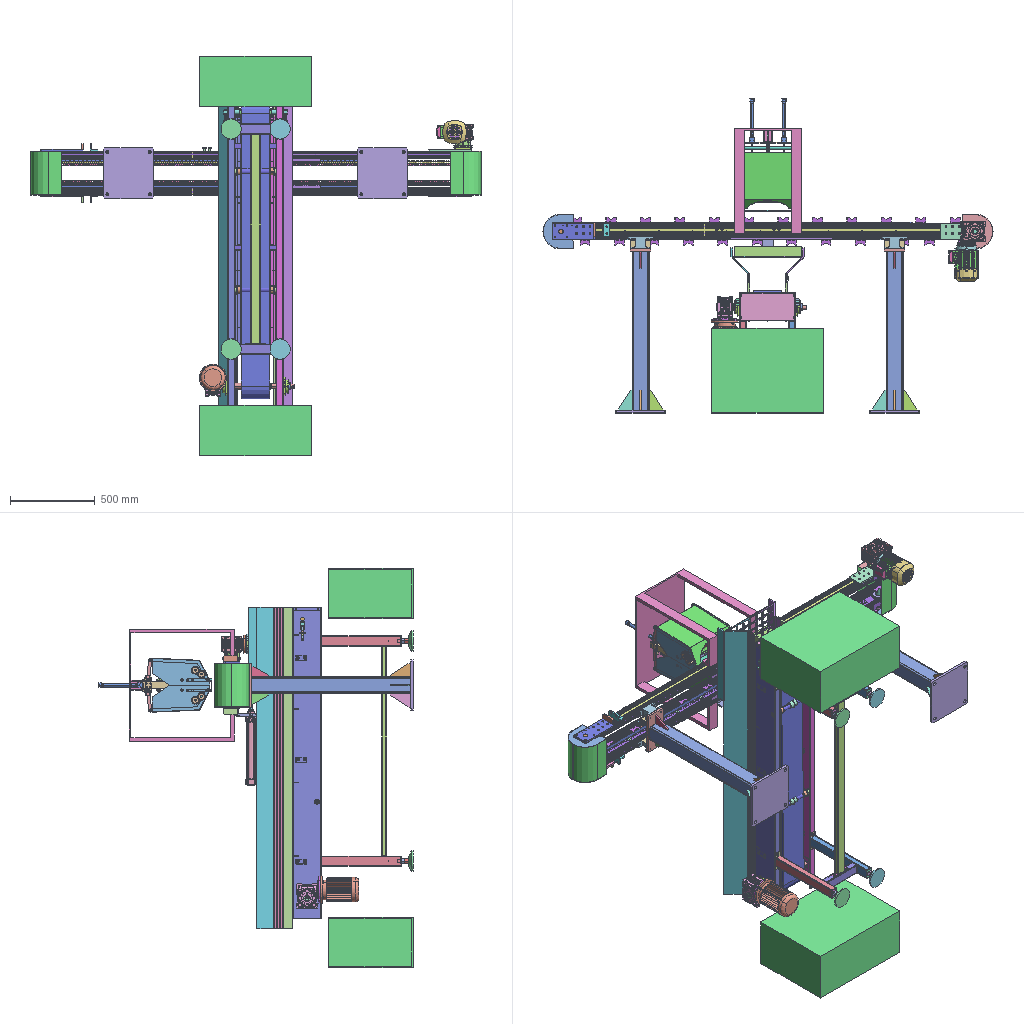Assembly | SolidWorks | 114 different items | 1113 placed | box 2658 x 1857 x 2360 mm
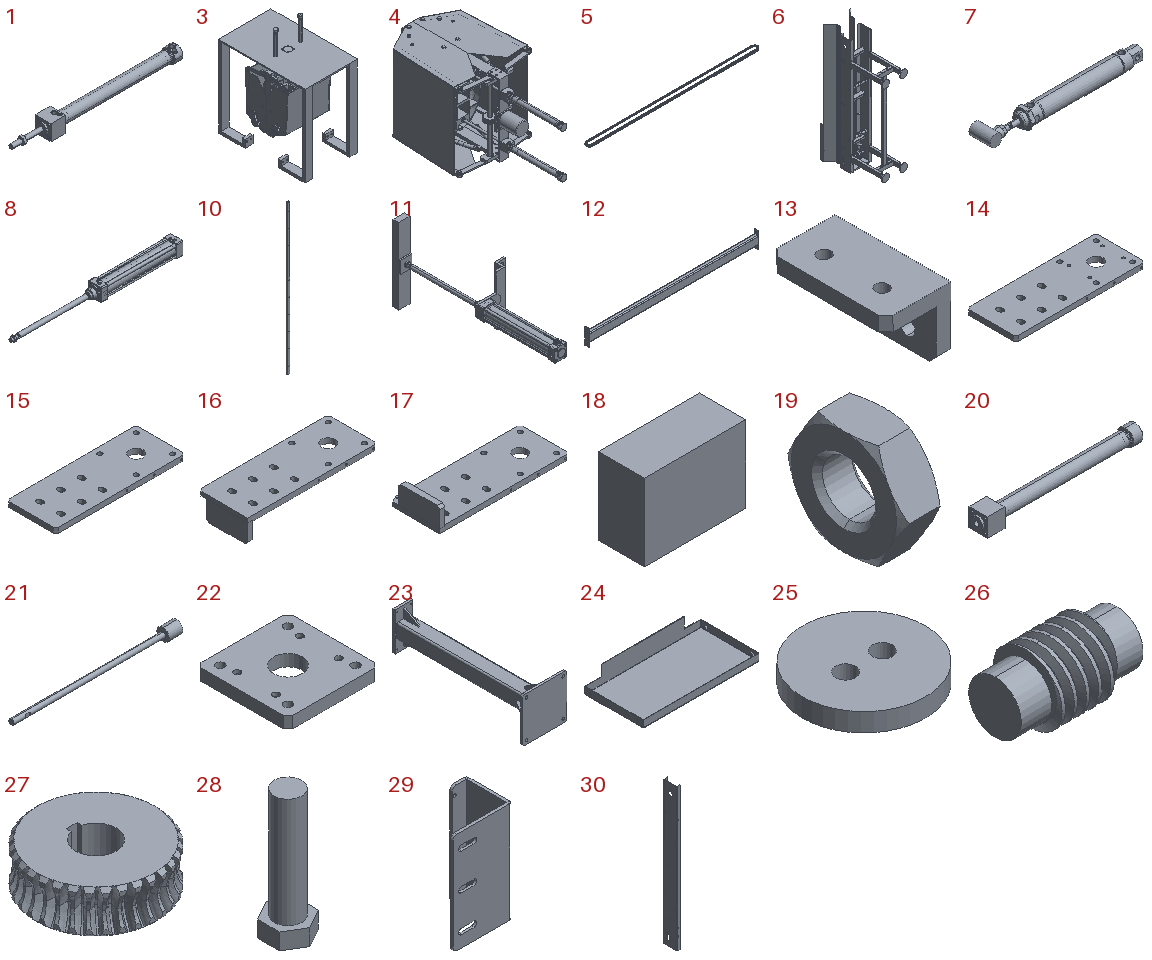Parts list (item | name | quantity | parent item | size | volume | features):
1 | (subassembly) | x2 | in 4 | 322.308 x 30.5 x 30.5 mm | 65420 mm3 | -
2 | (subassembly) | x1 | in 6 | - | - | -
3 | (subassembly) | x1 | - | - | 9842736 mm3 | -
4 | (subassembly) | x1 | in 3 | - | 3212108 mm3 | features CompositeCurve 13, ReferencePattern 9, MirrorCompFeat 4
5 | (subassembly) | x2 | - | - | 534431 mm3 | features ReferencePattern 402, LocalChainPattern 1
6 | (subassembly) | x1 | - | 432 x 974 x 1900 mm | 14530091 mm3 | features ReferencePattern 16, LocalLPattern 2, MirrorCompFeat 2
7 | (subassembly) | x4 | in 4 | 131.292 x 21.537 x 14.5 mm | 12191 mm3 | -
8 | (subassembly) | x1 | in 11 | 828.5 x 86 x 65 mm | 699915 mm3 | -
9 | (subassembly) | x2 | in 6 | - | - | -
10 | (subassembly) | x2 | - | 30 x 24 x 2000 mm | 1183134 mm3 | -
11 | (subassembly) | x1 | - | 190 x 856.5 x 400 mm | 1862385 mm3 | features CompositeCurve 1
12 | - | x1 | in 6 | 1240 x 30 x 120 mm | 613897 mm3 | features ICE 1, MirrorSolid 1, WeldMemberFeat 1, WeldmentFeature 1
13 | - | x2 | - | 45 x 80 x 45 mm | 60593 mm3 | features 3DProfileFeature 2, HoleWzd 2, Chamfer 1, Extrusion 1, LPattern 1
14 | - | x1 | - | 250 x 95 x 10 mm | 222392 mm3 | features 3DProfileFeature 4, HoleWzd 4, ICE 2, LPattern 2, Chamfer 1, Extrusion 1
15 | - | x1 | - | 250 x 95 x 10 mm | 223177 mm3 | features 3DProfileFeature 4, HoleWzd 4, ICE 2, LPattern 2, Chamfer 1, Extrusion 1
16 | - | x1 | - | 250 x 95 x 45 mm | 250777 mm3 | features 3DProfileFeature 4, HoleWzd 4, ICE 4, Chamfer 2, LPattern 2, Extrusion 1
17 | - | x1 | - | 250 x 95 x 45 mm | 250777 mm3 | features 3DProfileFeature 4, HoleWzd 4, ICE 4, Chamfer 2, LPattern 2, Extrusion 1
18 | - | x2 | - | 660 x 300 x 500 mm | 11192000 mm3 | features Extrusion 1, Shell 1
19 | - | x2 | in 1 | 5 x 15.011 x 13 mm | 543.306 mm3 | features BaseBody 1
20 | - | x2 | in 1 | 262 x 30.5 x 30.5 mm | 46248 mm3 | features BaseBody 1
21 | - | x2 | in 1 | 263 x 19.5 x 19.5 mm | 18628 mm3 | features BaseBody 1
22 | - | x1 | - | 95 x 95 x 12 mm | 92833 mm3 | features 3DProfileFeature 3, HoleWzd 3, Chamfer 1, Extrusion 1, ICE 1
23 | - | x2 | - | 300 x 970 x 300 mm | 3763524 mm3 | features Gusset 12, HoleWzd 4, ICE 4, 3DProfileFeature 2, Chamfer 2, MirrorPattern 1, WeldMemberFeat 1, WeldmentFeature 1
24 | - | x1 | in 6 | 324 x 164 x 50 mm | 116232 mm3 | features MoveCopyBody 4, Stock 4, Extrusion 1, FlatPattern 1, FlattenBends 1, ICE 1, ProcessBends 1, Rip 1, SMBaseFlange 1, SheetMetal 1, Shell 1
25 | - | x1 | - | 40 x 40 x 6 mm | 7142 mm3 | features Extrusion 1
26 | - | x1 | in 4 | 39.25 x 22.5 x 22.5 mm | 10547 mm3 | features ICE 2, Helix 1, RefAxis 1, Revolution 1, SweepCut 1
27 | - | x2 | in 4 | 45.721 x 45.721 x 15.75 mm | 18731 mm3 | features CirPattern 1, Cut 1, Helix 1, ICE 1, MirrorPattern 1, RefAxis 1, Revolution 1, SweepCut 1
28 | - | x4 | in 4 | 7.081 x 8.081 x 23 mm | 520.005 mm3 | features Extrusion 1, ICE 1
29 | - | x4 | - | 70 x 54 x 120 mm | 47871 mm3 | features 3DProfileFeature 1, Fillet 1, FlatPattern 1, HoleWzd 1, ICE 1, SMBaseFlange 1, SheetMetal 1
30 | - | x1 | in 6 | 100 x 170 x 1838 mm | 1266311 mm3 | features Cut 1, ICE 1, MirrorStock 1
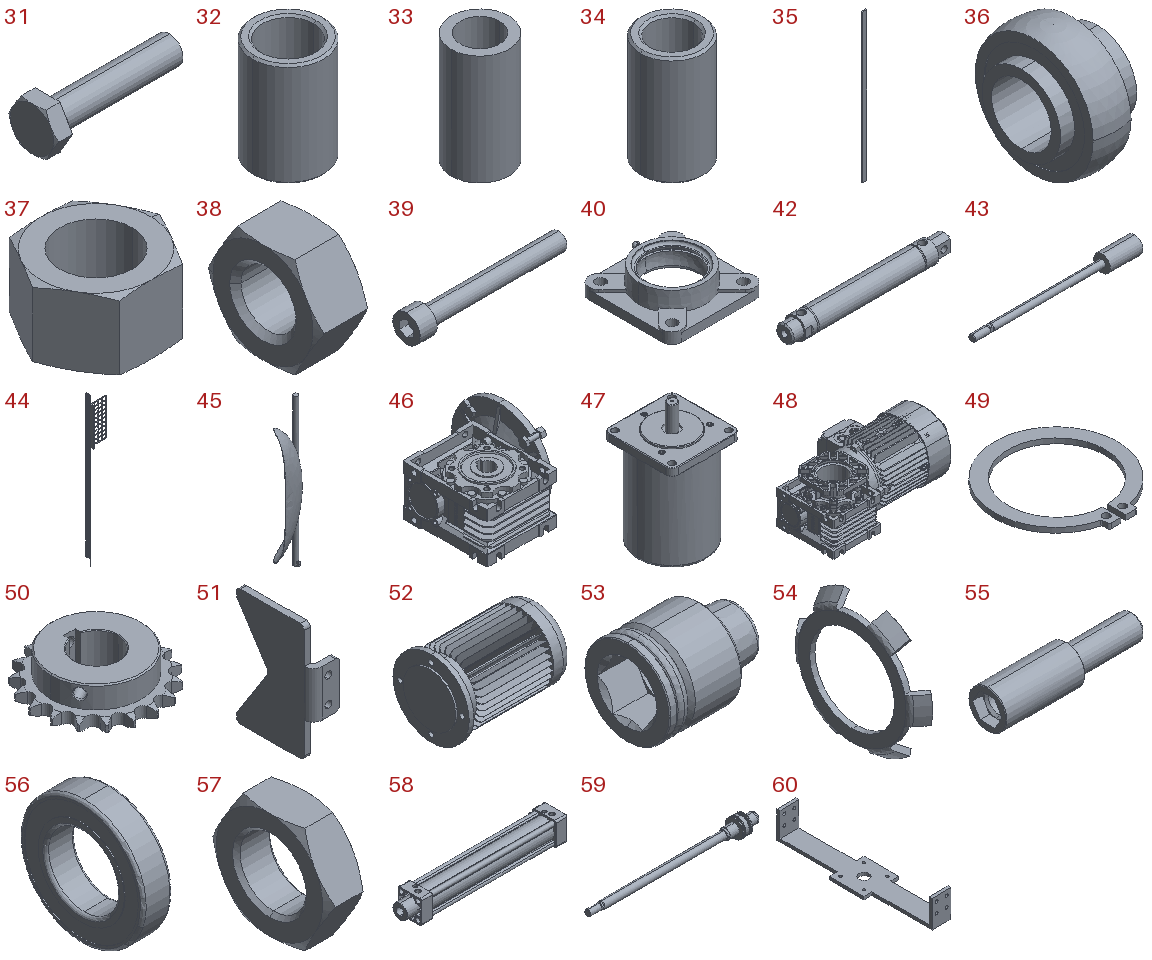31 | - | x4 | - | 51.4 x 18.475 x 16 mm | 4916 mm3 | features RevCut 3, Extrusion 1, Fillet 1, LPattern 1, Revolution 1
32 | - | x1 | in 6 | 35 x 35 x 51 mm | 22832 mm3 | features Chamfer 1, Extrusion 1
33 | - | x4 | in 6 | 30 x 30 x 57 mm | 21477 mm3 | features Chamfer 1, Extrusion 1
34 | - | x4 | in 6 | 30 x 30 x 52 mm | 19435 mm3 | features Chamfer 1, Extrusion 1
35 | - | x2 | - | 55 x 12 x 1900 mm | 1254000 mm3 | features Extrusion 1
36 | - | x2 | - | 38.1 x 62 x 62 mm | 38211 mm3 | features Revolution 3, RevCut 2, CirPattern 1
37 | - | x2 | in 6 | 17.59 x 15.233 x 9.5 mm | 1159 mm3 | features Cut 2, Chamfer 1, Extrusion 1
38 | - | x4 | in 7 | 3 x 6.928 x 6 mm | 65.89 mm3 | features RefAxis 3, 3DProfileFeature 1, ICE 1, Revolution 1, Scale 1
39 | - | x2 | in 6 | 90 x 16 x 16 mm | 8008 mm3 | features BlendCut 1, Cut 1, Fillet 1, LPattern 1, RevCut 1, Revolution 1
40 | - | x2 | - | 108 x 108 x 32.161 mm | 104974 mm3 | features Boss 2, Cut 1, Extrusion 1, RevCut 1, Revolution 1
41 | - | x4 | in 7 | - | - | features RefAxis 3, 3DProfileFeature 1
42 | - | x4 | in 7 | 102.5 x 13.5 x 13.5 mm | 7743 mm3 | features RefAxis 18, 3DProfileFeature 6, ICE 4, RevCut 2, Revolution 1, Scale 1
43 | - | x4 | in 7 | 97.25 x 10 x 10 mm | 2498 mm3 | features RefAxis 6, ICE 4, 3DProfileFeature 2, Revolution 1, Scale 1
44 | - | x1 | in 6 | 216 x 206 x 1900 mm | 3633510 mm3 | features MirrorStock 1
45 | - | x1 | in 4 | 71.359 x 45.899 x 361 mm | 54117 mm3 | features Attribute 3, MirrorStock 1
46 | - | x1 | - | 160 x 190.03 x 160.06 mm | 1157137 mm3 | features BaseBody 9
47 | - | x1 | in 4 | 57 x 57 x 99.8 mm | 207235 mm3 | features ICE 4, CirPattern 1, Fillet 1, LPattern 1, RevCut 1, Revolution 1, Sweep 1
48 | - | x1 | - | - | 1755237 mm3 | features MBimport 1
49 | - | x4 | - | 29.4 x 30.8 x 1.2 mm | 307.898 mm3 | features MBimport 1
50 | - | x4 | - | 83.793 x 83.51 x 22.064 mm | 58564 mm3 | features MBimport 1
51 | - | x39 | - | 13 x 38 x 58 mm | 5478 mm3 | features Fillet 2, ICE 2, FlatPattern 1, HoleWzd 1, SMBaseFlange 1, SheetMetal 1
52 | - | x1 | - | 228.5 x 160 x 160 mm | 2710519 mm3 | features CirPattern 2, ICE 2, Chamfer 1, Fillet 1, Revolution 1
53 | - | x2 | in 8 | 12.8 x 10 x 10 mm | 615.277 mm3 | features BaseBody 1
54 | - | x2 | in 8 | 1.224 x 10 x 9.485 mm | 14.031 mm3 | features BaseBody 1
55 | - | x8 | in 8 | 46 x 12 x 12 mm | 3091 mm3 | features BaseBody 1
56 | - | x8 | in 4 | 5 x 21 x 21 mm | 741.464 mm3 | features BaseBody 16
57 | - | x1 | in 8 | 8 x 26.558 x 23 mm | 2309 mm3 | features BaseBody 1
58 | - | x1 | in 8 | 436.5 x 86 x 65 mm | 489928 mm3 | features BaseBody 1
59 | - | x1 | in 8 | 465.5 x 49.5 x 49.5 mm | 181589 mm3 | features BaseBody 1
60 | - | x1 | in 4 | 70 x 312 x 55 mm | 103168 mm3 | features ICE 4, Cut 1, Extrusion 1
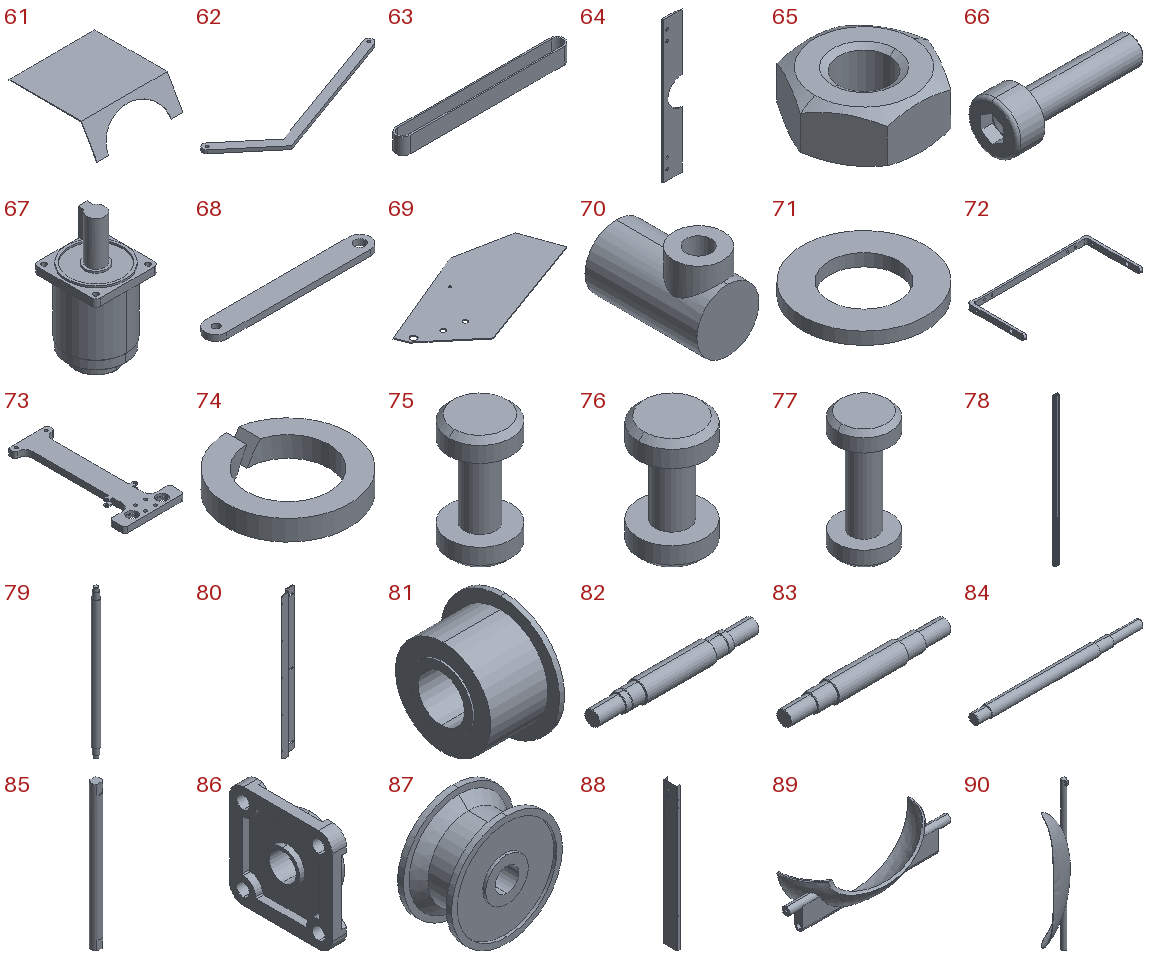61 | - | x2 | in 4 | 328 x 336.732 x 105.923 mm | 222158 mm3 | features Attribute 3, ICE 2, Extrusion 1
62 | - | x4 | in 4 | 377.416 x 116.677 x 7 mm | 52365 mm3 | features Extrusion 1, Fillet 1
63 | - | x1 | - | 1760 x 150 x 170 mm | 9292493 mm3 | features Extrusion 1
64 | - | x2 | in 4 | 37.5 x 3 x 280 mm | 23848 mm3 | features Cut 1, Extrusion 1, ICE 1
65 | - | x2 | - | 8.083 x 7 x 3.2 mm | 104.299 mm3 | features RevCut 2, Chamfer 1, Extrusion 1, LPattern 1
66 | - | x2 | - | 15 x 5.5 x 5.5 mm | 147.329 mm3 | features Fillet 2, RevCut 2, Boss 1, Chamfer 1, Cut 1, Extrusion 1, LPattern 1
67 | - | x2 | in 4 | 35 x 35 x 71 mm | 41626 mm3 | features ICE 7, Fillet 6, Revolution 5, Attribute 3, CirPattern 2, Extrusion 2, Chamfer 1, Dome 1, Emboss 1, LibraryFeature 1, Scale 1
68 | - | x4 | in 4 | 138 x 18 x 5 mm | 11613 mm3 | features ICE 2, Extrusion 1
69 | - | x4 | in 4 | 372.459 x 203.626 x 2 mm | 88439 mm3 | features Cut 6, ICE 4, Extrusion 1, Fillet 1
70 | - | x4 | in 7 | 10 x 18 x 13 mm | 1548 mm3 | features Extrusion 1, ICE 1
71 | - | x3 | - | 16 x 16 x 1.6 mm | 219.911 mm3 | features Extrusion 1
72 | - | x2 | in 4 | 314 x 149.984 x 15 mm | 51932 mm3 | features ICE 3, Fillet 2, Cut 1, Extrusion 1
73 | - | x2 | in 4 | 120 x 255 x 12 mm | 150718 mm3 | features ICE 8, Fillet 2, Cut 1, Extrusion 1
74 | - | x2 | - | 6.6 x 6.6 x 1.1 mm | 20.135 mm3 | features Cut 1, Extrusion 1
75 | - | x4 | in 4 | 12 x 12 x 22 mm | 1265 mm3 | features Chamfer 2, ICE 2, Extrusion 1
76 | - | x4 | in 4 | 12 x 12 x 20 mm | 1208 mm3 | features Chamfer 2, ICE 2, Extrusion 1
77 | - | x4 | in 4 | 12 x 12 x 27 mm | 1406 mm3 | features Chamfer 2, ICE 2, Extrusion 1
78 | - | x2 | - | 80 x 40 x 2300 mm | 2517050 mm3 | features MBimport 1
79 | - | x2 | in 4 | 15 x 15 x 320 mm | 52932 mm3 | features ICE 5, Chamfer 1, Extrusion 1, MirrorPattern 1
80 | - | x2 | - | 70 x 18 x 600 mm | 99365 mm3 | features 3DProfileFeature 1, Fillet 1, FlatPattern 1, HoleWzd 1, ICE 1, SMBaseFlange 1, SheetMetal 1
81 | - | x4 | in 6 | 27.5 x 51 x 51 mm | 16998 mm3 | features Revolution 1
82 | - | x1 | - | 276 x 35 x 35 mm | 204867 mm3 | features ICE 4, Chamfer 3, 3DProfileFeature 1, HoleWzd 1, MirrorPattern 1, Revolution 1
83 | - | x1 | - | 276 x 35 x 35 mm | 205103 mm3 | features Chamfer 1, ICE 1, Revolution 1
84 | - | x1 | - | 511 x 35 x 35 mm | 419085 mm3 | features ICE 2, Chamfer 1, HoleWzd 1, Revolution 1
85 | - | x1 | in 6 | 25 x 25 x 374 mm | 180094 mm3 | features ICE 2, Chamfer 1, Extrusion 1, MirrorPattern 1
86 | - | x4 | - | 35.7 x 95 x 95 mm | 103360 mm3 | features MBimport 1
87 | - | x4 | in 6 | 117 x 57 x 117 mm | 342775 mm3 | features ICE 2, MirrorPattern 1, Revolution 1
88 | - | x1 | in 6 | 100 x 170 x 1838 mm | 1271220 mm3 | features ICE 5, MoveCopyBody 4, Stock 4, FlatPattern 2, SMBaseFlange 2, SheetMetal 2, Chamfer 1, HoleWzd 1, LPattern 1, RefAxis 1, SMMiteredFlange 1
89 | - | x2 | in 4 | 328 x 89.443 x 98.481 mm | 199314 mm3 | features ICE 3, MirrorPattern 2, 3DProfileFeature 1, Attribute 1, Chamfer 1, Revolution 1
90 | - | x1 | in 4 | 71.359 x 45.899 x 361 mm | 54038 mm3 | features ICE 4, Attribute 3, Cut 3, Chamfer 2, ExtruThin 1, Fillet 1, Shell 1, Sweep 1
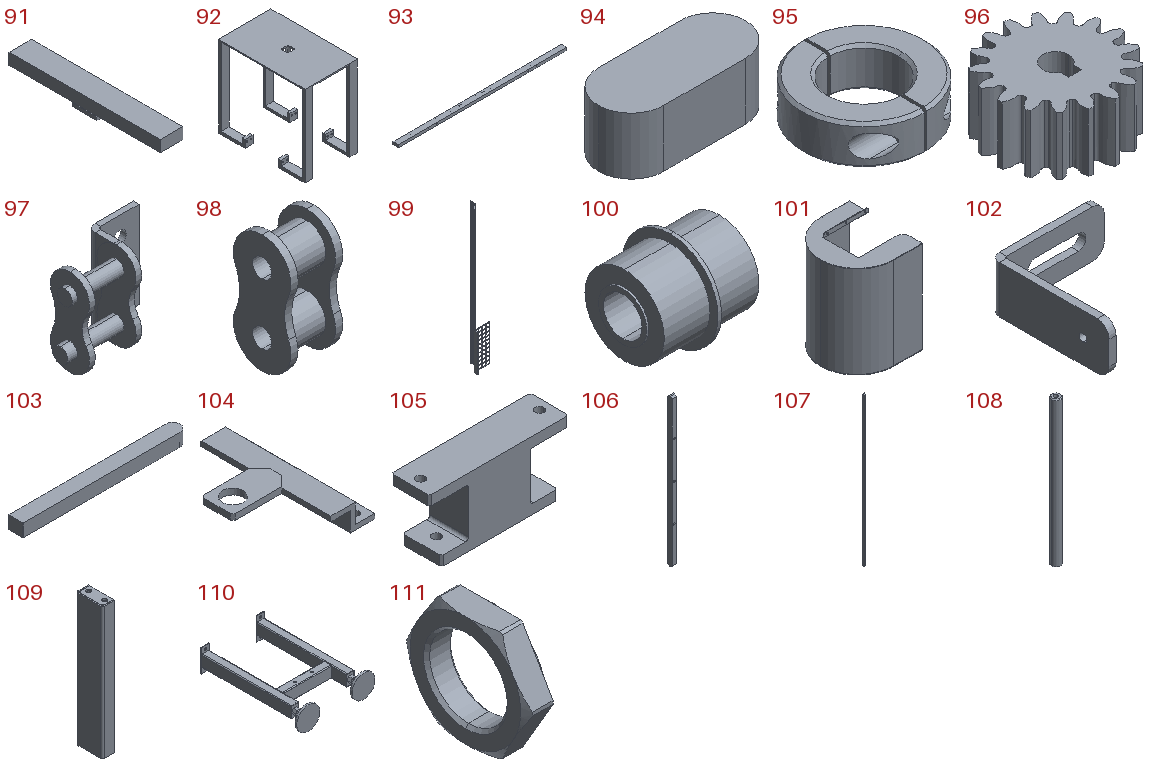91 | - | x1 | in 11 | 60 x 400 x 40 mm | 758635 mm3 | features Cut 2, ICE 2, Chamfer 1, Extrusion 1, HoleWzd 1
92 | - | x1 | in 3 | 400 x 660 x 620 mm | 6630473 mm3 | features MirrorPattern 6, ICE 5, Cut 1, Extrusion 1
93 | - | x2 | - | 2544 x 80 x 40 mm | 8091371 mm3 | features Cut 4, Extrusion 1, LPattern 1
94 | - | x4 | - | 18 x 8 x 7 mm | 911.858 mm3 | features MBimport 1
95 | - | x2 | in 6 | 44 x 43.989 x 14 mm | 11608 mm3 | features ICE 3, Chamfer 1, Extrusion 1, MirrorSolid 1
96 | - | x4 | in 4 | 47.423 x 47.235 x 22.5 mm | 29237 mm3 | features Attribute 3, ICE 2, CirPattern 1, Cut 1, Extrusion 1, RefAxis 1, Scale 1
97 | - | x404 | in 5 | 27.296 x 13.105 x 23.11 mm | 1387 mm3 | features MoveFace 9, 3DProfileFeature 1, BaseBody 1, EdgeFlange 1, FlatPattern 1, HoleWzd 1, SMBaseFlange 1, SheetMetal 1
98 | - | x404 | in 5 | 10.85 x 12.07 x 24.77 mm | 1258 mm3 | features MoveFace 4, BaseBody 1, DelFace 1
99 | - | x1 | in 6 | 216 x 206 x 1900 mm | 3633510 mm3 | features ICE 5, Cut 1, Extrusion 1, LPattern 1
100 | - | x2 | in 6 | 51 x 49.5 x 49.5 mm | 50740 mm3 | features Revolution 1
101 | - | x2 | - | 182 x 204 x 280 mm | 308459 mm3 | features FlatPattern 3, SMBaseFlange 2, SheetMetal 2, 3DProfileFeature 1, EdgeFlange 1, Fillet 1, HoleWzd 1, MirrorSolid 1
102 | - | x20 | - | 45 x 50 x 20 mm | 4913 mm3 | features 3DProfileFeature 1, Fillet 1, FlatPattern 1, HoleWzd 1, ICE 1, SMBaseFlange 1, SheetMetal 1
103 | - | x1 | - | 90 x 8 x 7 mm | 4991 mm3 | features MBimport 1
104 | - | x1 | in 11 | 190 x 265 x 52 mm | 403840 mm3 | features ICE 4, Chamfer 2, Extrusion 1
105 | - | x4 | - | 144 x 40 x 70 mm | 231204 mm3 | features ICE 4, 3DProfileFeature 3, HoleWzd 3, Cut 2, Chamfer 1, Extrusion 1, Fillet 1, MirrorPattern 1
106 | - | x4 | - | 6 x 6 x 200 mm | 7064 mm3 | features 3DProfileFeature 1, Chamfer 1, Extrusion 1, HoleWzd 1
107 | - | x2 | - | 6 x 6 x 600 mm | 21405 mm3 | features 3DProfileFeature 1, Chamfer 1, Extrusion 1, HoleWzd 1
108 | - | x2 | in 6 | 20 x 20 x 324 mm | 98619 mm3 | features HoleWzd 2, Chamfer 1, Extrusion 1
109 | - | x3 | in 6 | 30 x 65 x 324 mm | 129406 mm3 | features MoveCopyBody 5, Stock 5, FlatPattern 2, SMBaseFlange 2, SheetMetal 2, ICE 1, MirrorSolid 1
110 | - | x2 | in 6 | 410 x 543 x 120 mm | 1073407 mm3 | features MoveCopyBody 4, Stock 4, ICE 3, WeldMemberFeat 2, HoleWzd 1, MirrorSolid 1, WeldCornerFeat 1, WeldmentFeature 1
111 | - | x4 | in 7 | 3.5 x 16.5 x 14.5 mm | 336.894 mm3 | features RefAxis 6, 3DProfileFeature 2, ICE 1, RevCut 1, Revolution 1, Scale 1
112 | VSW26-40-L2000-K10-P200.stp (subassembly) | x1 | - | - | - | -
113 | _VSW26-40                                                        40 2000 10 200 VSW26.stp | x1 | - | - | - | -
114 | _VSW26-L2000                                                        40 2000 10 200 VSW26.stp | x1 | - | - | - | -
Mates (type | each side: item.copy, entity, surface, feature), first 366 of 395 lines:
In the top assembly
Coincident | 23.1 face plane Boss-Extrude 1 | 23.2 face plane Boss-Extrude 1
Coincident | 23.1 face plane Square Tube 100 X 100 X 5(1) | 23.2 face plane Square Tube 100 X 100 X 5(1)
DistanceDim | 23.2 face plane Square Tube 100 X 100 X 5(1) | 23.1 face plane Square Tube 100 X 100 X 5(1)
Concentric | 105.1 face cylinder M8 Clearance Hole 1 | 23.1 face cylinder M8 Tapped Hole 1 | 2 times
Coincident | 105.1 face plane Boss-Extrude 1 | 23.1 face plane Boss-Extrude 2
Concentric | 23.1 face cylinder M8 Tapped Hole 1 | 105.2 face cylinder M8 Clearance Hole 1 | 2 times
Coincident | 23.1 face plane Boss-Extrude 2 | 105.2 face plane Boss-Extrude 1
Concentric | 23.2 face cylinder M8 Tapped Hole 1 | 105.3 face cylinder M8 Clearance Hole 1 | 2 times
Coincident | 23.2 face plane Boss-Extrude 2 | 105.3 face plane Boss-Extrude 1
Concentric | 23.2 face cylinder M8 Tapped Hole 1 | 105.4 face cylinder M8 Clearance Hole 1 | 2 times
Coincident | 23.2 face plane Boss-Extrude 2 | 105.4 face plane Boss-Extrude 1
Coincident | 105.1 face plane Boss-Extrude 1 | 78.1 face plane AOB05-4080E-L2300.stp
Coincident | 78.2 face plane AOB05-4080E-L2300.stp | 78.1 face plane AOB05-4080E-L2300.stp | 2 times
Width | 78.1 face plane AOB05-4080E-L2300.stp | 78.1 face plane AOB05-4080E-L2300.stp | 105.1 face plane Boss-Extrude 1 | 105.1 face plane Boss-Extrude 1
Width | 78.2 face plane AOB05-4080E-L2300.stp | 78.2 face plane AOB05-4080E-L2300.stp | 105.2 face plane Boss-Extrude 1 | 105.2 face plane Boss-Extrude 1
Width | 78.2 face plane AOB05-4080E-L2300.stp | 78.2 face plane AOB05-4080E-L2300.stp | 23.1 face plane Square Tube 100 X 100 X 5(1) | 23.2 face plane Square Tube 100 X 100 X 5(1)
Coincident | 15.1 face plane Boss-Extrude 1 | 78.2 face plane AOB05-4080E-L2300.stp | 2 times
Concentric | 15.1 face cylinder Cut-Extrude 5 | 86.1 face cylinder BDR-205.stp
Coincident | 15.1 face plane Boss-Extrude 1 | 86.1 face plane BDR-205.stp
Width | 78.1 face plane AOB05-4080E-L2300.stp | 78.2 face plane AOB05-4080E-L2300.stp | 50.1 face plane VLF02-40-19-D30.stp | 50.2 face plane VLF02-40-19-D30.stp
Concentric | 86.1 face cylinder BDR-205.stp | 83.1 face cylinder Revolve 1 | 2 times
Coincident | 83.1 face plane Revolve 1 | 50.2 face plane VLF02-40-19-D30.stp
Concentric | 83.1 face cylinder Revolve 1 | 50.2 face cylinder VLF02-40-19-D30.stp
Concentric | 83.1 face cylinder Revolve 1 | 50.1 face cylinder VLF02-40-19-D30.stp
Coincident | 83.1 face plane Revolve 1 | 50.1 face plane VLF02-40-19-D30.stp
Concentric | 83.1 face cylinder Cut-Extrude 1 | 94.1 face cylinder BLC01-B8-L18.stp
Coincident | 83.1 face plane Cut-Extrude 1 | 94.1 face plane BLC01-B8-L18.stp | 2 times
Concentric | 83.1 face cylinder Cut-Extrude 1 | 94.2 face cylinder BLC01-B8-L18.stp
Coincident | 83.1 face plane Cut-Extrude 1 | 94.2 face plane BLC01-B8-L18.stp | 2 times
Coincident | 50.2 face plane VLF02-40-19-D30.stp | 94.2 face plane BLC01-B8-L18.stp
Coincident | 50.1 face plane VLF02-40-19-D30.stp | 94.1 face plane BLC01-B8-L18.stp
DistanceDim | 15.1 face plane Boss-Extrude 1 | 78.2 face plane AOB05-4080E-L2300.stp
Coincident | 78.1 face plane AOB05-4080E-L2300.stp | 14.1 face plane Boss-Extrude 1 | 2 times
Coincident | 15.1 face plane Boss-Extrude 1 | 14.1 face plane Boss-Extrude 1
Concentric | 86.2 face cylinder BDR-205.stp | 14.1 face cylinder Cut-Extrude 5
Coincident | 86.2 face plane BDR-205.stp | 14.1 face plane Boss-Extrude 1
Concentric | 22.1 face cylinder Cut-Extrude 1 | 14.1 face cylinder Cut-Extrude 5
Coincident | 22.1 face plane Boss-Extrude 1 | 14.1 face plane Boss-Extrude 1
Parallel | 22.1 face plane Boss-Extrude 1 | 14.1 face plane Boss-Extrude 1
Coincident | 78.1 face plane AOB05-4080E-L2300.stp | 17.1 face plane Boss-Extrude 1 | 2 times
DistanceDim | 17.1 face plane Boss-Extrude 1 | 78.1 face plane AOB05-4080E-L2300.stp
Coincident | 78.2 face plane AOB05-4080E-L2300.stp | 16.1 face plane Boss-Extrude 1 | 2 times
Coincident | 17.1 face plane Boss-Extrude 1 | 16.1 face plane Boss-Extrude 1
Coincident | 13.1 face plane Boss-Extrude 1 | 78.1 face plane AOB05-4080E-L2300.stp | 2 times
DistanceDim | 13.1 face plane Boss-Extrude 1 | 17.1 face plane Boss-Extrude 1
Concentric | 17.1 face cylinder Cut-Extrude 5 | 86.3 face cylinder BDR-205.stp
Coincident | 17.1 face plane Boss-Extrude 1 | 86.3 face plane BDR-205.stp
Coincident | 16.1 face plane Boss-Extrude 1 | 86.4 face plane BDR-205.stp
Concentric | 16.1 face cylinder Cut-Extrude 5 | 86.4 face cylinder BDR-205.stp
Concentric | 86.4 face cylinder BDR-205.stp | 82.1 face cylinder Revolve 1
Concentric | 82.1 face cylinder Revolve 1 | 50.3 face cylinder VLF02-40-19-D30.stp
Concentric | 82.1 face cylinder Revolve 1 | 50.4 face cylinder VLF02-40-19-D30.stp
Concentric | 82.1 face cylinder Cut-Extrude 1 | 94.3 face cylinder BLC01-B8-L18.stp
Coincident | 82.1 face plane Cut-Extrude 1 | 94.3 face plane BLC01-B8-L18.stp
Concentric | 82.1 face cylinder Cut-Extrude 1 | 94.4 face cylinder BLC01-B8-L18.stp
Coincident | 82.1 face plane Cut-Extrude 1 | 94.4 face plane BLC01-B8-L18.stp
Coincident | 82.1 face plane Revolve 1 | 50.3 face plane VLF02-40-19-D30.stp
Coincident | 82.1 face plane Revolve 1 | 50.4 face plane VLF02-40-19-D30.stp
Width | 50.3 face plane VLF02-40-19-D30.stp | 50.4 face plane VLF02-40-19-D30.stp | 78.1 face plane AOB05-4080E-L2300.stp | 78.2 face plane AOB05-4080E-L2300.stp
Concentric | 50.4 face cylinder VLF02-40-19-D30.stp | 5.1 select_type:24
Width | 98.1 face plane Import 1 | 98.1 face plane Import 1 | 50.4 face plane VLF02-40-19-D30.stp | 50.4 face plane VLF02-40-19-D30.stp
Concentric | 50.2 face cylinder VLF02-40-19-D30.stp | 5.2 select_type:24
Coincident | 97.1 face plane Edge-Flange 1 | 51.1 face plane Base-Flange 1
Parallel | 78.2 face plane AOB05-4080E-L2300.stp | 5.2 select_type:24
Width | 98.2 face plane Import 1 | 98.2 face plane Import 1 | 50.3 face plane VLF02-40-19-D30.stp | 50.3 face plane VLF02-40-19-D30.stp
Parallel | 78.1 face plane AOB05-4080E-L2300.stp | 5.1 select_type:24
Concentric | 97.2 face cylinder Ø3.4 (3.4) DiameterHole 1 | 51.2 face cylinder Ø3.4 (3.4) DiameterHole 1 | 2 times
Coincident | 97.2 face plane Edge-Flange 1 | 51.2 face plane Base-Flange 1
Concentric | 97.3 face cylinder Ø3.4 (3.4) DiameterHole 1 | 51.3 face cylinder Ø3.4 (3.4) DiameterHole 1 | 2 times
Coincident | 97.3 face plane Edge-Flange 1 | 51.3 face plane Base-Flange 1
Coincident | 29.1 face plane Base-Flange 1 | 23.1 face plane Boss-Extrude 2
Width | 29.1 face plane Base-Flange 1 | 29.1 face plane Base-Flange 1 | 23.1 face plane Boss-Extrude 2 | 23.1 face plane Boss-Extrude 2
Coincident | 29.1 face plane Base-Flange 1 | 29.2 face plane Base-Flange 1 | 2 times
Width | 29.2 face plane Base-Flange 1 | 29.1 face plane Base-Flange 1 | 23.1 face plane Boss-Extrude 2 | 23.1 face plane Boss-Extrude 2
Coincident | 29.3 face plane Base-Flange 1 | 29.4 face plane Base-Flange 1 | 2 times
Coincident | 23.2 face plane Boss-Extrude 2 | 29.3 face plane Base-Flange 1
Coincident | 16.1 face plane Boss-Extrude 1 | 101.1 face plane Mirror 1
DistanceDim | 16.1 face plane Boss-Extrude 1 | 101.1 face plane Mirror 1
Width | 101.1 face plane Mirror 1 | 101.1 face plane Base-Flange 2 | 17.1 face plane Boss-Extrude 1 | 16.1 face plane Boss-Extrude 1
Coincident | 14.1 face plane Boss-Extrude 1 | 101.2 face plane Mirror 1
DistanceDim | 14.1 face plane Boss-Extrude 1 | 101.2 face plane Mirror 1
Coincident | 101.2 face plane Mirror 1 | 101.1 face plane Base-Flange 2
Concentric | 22.1 face cylinder Cut-Extrude 1 | 48.1 face cylinder NMRW050-MS7124-B14-FA1-D25.STEP
Parallel | 22.1 face plane Boss-Extrude 1 | 48.1 face plane NMRW050-MS7124-B14-FA1-D25.STEP
Coincident | 22.1 face plane Boss-Extrude 1 | 48.1 face plane NMRW050-MS7124-B14-FA1-D25.STEP
Coincident | 97.4 face plane Edge-Flange 1 | 51.4 face plane Base-Flange 1
Concentric | 97.1 face cylinder Ø3.4 (3.4) DiameterHole 1 | 51.1 face cylinder Ø3.4 (3.4) DiameterHole 1 | 2 times
Concentric | 97.5 face cylinder Ø3.4 (3.4) DiameterHole 1 | 51.4 face cylinder Ø3.4 (3.4) DiameterHole 1 | 2 times
Coincident | 78.2 face plane AOB05-4080E-L2300.stp | 13.2 face plane Boss-Extrude 1
Coincident | 13.1 face plane Boss-Extrude 1 | 13.2 face plane Boss-Extrude 1
Concentric | 82.1 face cylinder Mirror 1 | 49.1 face cylinder TBP01-25.stp
Coincident | 82.1 face plane Mirror 1 | 49.1 face plane TBP01-25.stp
Concentric | 82.1 face cylinder Cut-Extrude 3 | 49.2 face cylinder TBP01-25.stp
Coincident | 82.1 face plane Cut-Extrude 3 | 49.2 face plane TBP01-25.stp
Concentric | 97.6 face cylinder Ø3.4 (3.4) DiameterHole 1 | 51.5 face cylinder Ø3.4 (3.4) DiameterHole 1 | 2 times
Coincident | 97.6 face plane Edge-Flange 1 | 51.5 face plane Base-Flange 1
Concentric | 97.7 face cylinder Ø3.4 (3.4) DiameterHole 1 | 51.6 face cylinder Ø3.4 (3.4) DiameterHole 1 | 2 times
Coincident | 97.7 face plane Edge-Flange 1 | 51.6 face plane Base-Flange 1
Coincident | 78.1 face plane AOB05-4080E-L2300.stp | 102.1 face plane Base-Flange 1
Coincident | 78.2 face plane AOB05-4080E-L2300.stp | 102.2 face plane Base-Flange 1
Coincident | 29.1 face plane Base-Flange 1 | 106.1 face plane Boss-Extrude 1 | 2 times
Concentric | 29.1 face cylinder M3 Clearance Hole 1 | 106.1 face cylinder M3 Tapped Hole 1
Coincident | 29.2 face plane Base-Flange 1 | 106.2 face plane Boss-Extrude 1 | 2 times
Concentric | 29.2 face cylinder M3 Clearance Hole 1 | 106.2 face cylinder M3 Tapped Hole 1
Width | 106.1 face plane Boss-Extrude 1 | 106.1 face plane Boss-Extrude 1 | 98.3 face plane Import 1 | 98.3 face plane Import 1
Coincident | 29.3 face plane Base-Flange 1 | 106.3 face plane Boss-Extrude 1 | 2 times
Concentric | 29.3 face cylinder M3 Clearance Hole 1 | 106.3 face cylinder M3 Tapped Hole 1
Coincident | 29.4 face plane Base-Flange 1 | 106.4 face plane Boss-Extrude 1 | 2 times
Concentric | 29.4 face cylinder M3 Clearance Hole 1 | 106.4 face cylinder M3 Tapped Hole 1
Coincident | 29.1 face plane Base-Flange 1 | 29.3 face plane Base-Flange 1
Width | 29.3 face plane Base-Flange 1 | 29.3 face plane Base-Flange 1 | 23.2 face plane Boss-Extrude 2 | 23.2 face plane Boss-Extrude 2
Coincident | 29.2 face plane Base-Flange 1 | 29.4 face plane Base-Flange 1
Coincident | 80.1 face plane Base-Flange 1 | 107.1 face plane Boss-Extrude 1 | 2 times
Concentric | 80.1 face cylinder M3 Clearance Hole 1 | 107.1 face cylinder M3 Tapped Hole 1
Coincident | 78.2 face plane AOB05-4080E-L2300.stp | 80.1 face plane Base-Flange 1
Coincident | 106.4 face plane Boss-Extrude 1 | 107.1 face plane Boss-Extrude 1
Coincident | 80.2 face plane Base-Flange 1 | 107.2 face plane Boss-Extrude 1 | 2 times
Concentric | 80.2 face cylinder M3 Clearance Hole 1 | 107.2 face cylinder M3 Tapped Hole 1
Coincident | 80.1 face plane Base-Flange 1 | 80.2 face plane Base-Flange 1 | 2 times
Coincident | 106.3 face plane Boss-Extrude 1 | 107.2 face plane Boss-Extrude 1
Concentric | 105.1 face cylinder Mirror 2 | 71.1 face cylinder Base-Extrude
Coincident | 105.1 face plane Cut-Extrude 2 | 71.1 face plane Base-Extrude
Concentric | 105.1 face cylinder Mirror 2 | 74.1 face cylinder Base-Extrude
Coincident | 71.1 face plane Base-Extrude | 74.1 face plane Base-Extrude
Concentric | 51.7 face cylinder Ø3.4 (3.4) DiameterHole 1 | 71.2 face cylinder Base-Extrude
Coincident | 51.7 face plane Base-Flange 1 | 71.2 face plane Base-Extrude
Concentric | 51.7 face cylinder Ø3.4 (3.4) DiameterHole 1 | 74.2 face cylinder Base-Extrude
Coincident | 71.2 face plane Base-Extrude | 74.2 face plane Base-Extrude
Coincident | 51.7 face plane Base-Flange 1 | 65.1 face plane BaseNut
Concentric | 74.2 face cylinder Base-Extrude | 65.2 face cone EndChamfer
Coincident | 74.2 face plane Base-Extrude | 65.2 face plane BaseNut
Concentric | 51.7 face cylinder Base Bend 1 | 66.1 face cylinder BaseBody
Concentric | 51.7 face cylinder Ø3.4 (3.4) DiameterHole 1 | 66.2 face cylinder BaseBody
Coincident | 71.3 face plane Base-Extrude | 66.2 face plane BaseHead
Coincident | 97.8 face plane Edge-Flange 1 | 71.3 face plane Base-Extrude
Concentric | 66.2 face cylinder BaseHead | 71.3 face cylinder Base-Extrude
Coincident | 102.3 face plane Base-Flange 1 | 93.1 face plane Boss-Extrude 1
Coincident | 102.1 face plane Base-Flange 1 | 93.1 face plane Boss-Extrude 1 | 2 times
Coincident | 101.1 face plane Base-Flange 2 | 93.1 face plane Boss-Extrude 1
Coincident | 23.2 face plane Boss-Extrude 1 | 110.1 face plane M20 Foot | 2 times
Coincident | 23.1 face plane Boss-Extrude 1 | 18.1 face plane Boss-Extrude 1
Parallel | 24.1 face plane Boss-Extrude 1 | 18.1 face plane Boss-Extrude 1
DistanceDim | 110.1 face plane Structure Member 1 | 18.1 face plane Boss-Extrude 1
Concentric | 84.1 face cylinder Revolve 1 | 36.1 face sphere Boss-Revolve 3
Concentric | 84.1 face cylinder Revolve 1 | 40.1 edge
Coincident | 88.1 face plane Base-Flange 1 | 40.1 face plane Base-Extrude
Concentric | 84.1 face cylinder Revolve 1 | 36.2 face cylinder Boss-Revolve 3
Coincident | 40.1 face plane Cut-Revolve 1 | 36.2 face plane Boss-Revolve 3
Concentric | 84.1 face cylinder Revolve 1 | 46.1 edge
Parallel | 88.1 face plane Base-Flange 1 | 46.1 face plane Import 1
Coincident | 46.1 face plane Import 7 | 25.1 face plane Boss-Extrude 1
Concentric | 46.1 edge | 25.1 edge
Concentric | 46.1 edge | 52.1 face cylinder Revolve 1
Concentric | 46.1 face cylinder Import 9 | 52.1 edge
Coincident | 46.1 face plane Import 9 | 52.1 face plane Revolve 1
DistanceDim | 84.1 face plane Revolve 1 | 36.1 face plane Boss-Revolve 3
Width | 18.1 face plane Boss-Extrude 1 | 18.1 face plane Boss-Extrude 1 | 30.1 face plane Side Beam 3 Mirror | 88.1 face plane Base-Flange 1
Concentric | 84.1 face cylinder Revolve 1 | 87.1 face cylinder Cut-Extrude 1
Coincident | 87.2 face plane Revolve 1 | 87.1 face plane Revolve 1
Concentric | 84.1 face cylinder Revolve 1 | 87.3 edge
Coincident | 87.4 face plane Revolve 1 | 87.3 face plane Revolve 1
Concentric | 30.1 edge | 84.1 face cylinder Revolve 1
Concentric | 84.1 face cylinder Revolve 1 | 40.2 edge
Coincident | 30.1 face plane Side Beam 3 Mirror | 40.2 face plane Base-Extrude
Parallel | 30.1 face plane Side Beam 3 Mirror | 40.2 face plane Base-Extrude
Concentric | 84.1 face cylinder Revolve 1 | 63.1 edge
Width | 63.1 face plane Boss-Extrude 1 | 63.1 face plane Boss-Extrude 1 | 30.1 face plane Side Beam 3 Mirror | 88.1 face plane Base-Flange 1
Coincident | 44.1 face plane Large C Type Guardrail_Mirror | 35.1 face plane Boss-Extrude 1 | 3 times
Coincident | 99.1 face plane Boss-Extrude 2 | 35.2 face plane Boss-Extrude 1 | 2 times
Coincident | 35.1 face plane Boss-Extrude 1 | 35.2 face plane Boss-Extrude 1
Width | 92.1 face plane Boss-Extrude 1 | 92.1 face plane Boss-Extrude 1 | 101.2 face plane Mirror 1 | 101.1 face plane Base-Flange 2
Width | 92.1 face plane Boss-Extrude 1 | 92.1 face plane Boss-Extrude 1 | 17.1 face plane Boss-Extrude 1 | 16.1 face plane Boss-Extrude 1
Width | 23.2 face plane Square Tube 100 X 100 X 5(1) | 23.1 face plane Square Tube 100 X 100 X 5(1) | 88.1 face plane Base-Flange 1 | 30.1 face plane Side Beam 3 Mirror
Coincident | 102.1 face plane Base-Flange 1 | 102.2 face plane Base-Flange 1
DistanceDim | 102.2 face plane Base-Flange 1 | 15.1 face plane Boss-Extrude 1
Width | 104.1 face plane Boss-Extrude 2 | 104.1 face plane Boss-Extrude 2 | 92.1 face plane Boss-Extrude 1 | 92.1 face plane Boss-Extrude 1
Coincident | 78.2 face plane AOB05-4080E-L2300.stp | 104.1 face plane Boss-Extrude 3
Coincident | 44.1 face plane Large C Type Guardrail_Mirror | 91.1 face plane Boss-Extrude 2
Coincident | 36.1 face plane Boss-Revolve 3 | 40.2 face plane Boss-Extrude 2
DistanceDim | 40.1 face plane Boss-Extrude 2 | 46.1 face plane Import 7
In subassembly 6
Concentric | 110.2 face cylinder Cut-Extrude 1 | 12.1 face cylinder Boss-Extrude 1
Coincident | 110.2 face plane Structure Member 2 | 12.1 face plane Boss-Extrude 1
Coincident | 110.3 face plane Structure Member 2 | 12.1 face plane Mirror 1
Concentric | 110.3 face cylinder Cut-Extrude 1 | 12.1 face cylinder Mirror 1 | 2 times
Concentric | 110.3 face cylinder Boss-Extrude 1 | 88.2 face cylinder GB/T41-20001 Type Hex Nut C Grade M102
Concentric | 110.2 face cylinder Boss-Extrude 1 | 88.2 face cylinder GB/T41-20001 Type Hex Nut C Grade M10
Coincident | 110.2 face plane Boss-Extrude 1 | 88.2 face plane Base-Flange 1
Concentric | 30.2 face cylinder Side Beam 3 Mirror | 109.1 face cylinder Mirror 1 | 2 times
Width | 109.1 face plane Mirror 1 | 109.1 face plane Base-Flange 2 | 88.2 face plane Base-Flange 1 | 30.2 face plane Side Beam 3 Mirror
Concentric | 88.2 axis | 85.1 face cylinder Boss-Extrude 1
Width | 88.2 face plane Base-Flange 1 | 30.2 face plane Side Beam 3 Mirror | 85.1 face plane Boss-Extrude 1 | 85.1 face plane Boss-Extrude 1
Width | 85.1 face plane Cut-Extrude 1 | 85.1 face plane Mirror 1 | 30.2 face plane Side Beam 3 Mirror | 30.2 face plane Side Beam 3 Mirror
Concentric | 85.1 face cylinder Boss-Extrude 1 | 87.5 face cylinder Cut-Extrude 1
Concentric | 88.2 face cylinder Cut-Extrude 1 | 24.2 face cylinder Cut-Extrude 1 | 2 times
Width | 88.2 face plane Base-Flange 1 | 30.2 face plane Side Beam 3 Mirror | 24.2 face plane Boss-Extrude 1 | 24.2 face plane Boss-Extrude 1
Concentric | 88.2 face cylinder Cut-Extrude 1 | 108.1 face cylinder Boss-Extrude 1
Width | 108.1 face plane Boss-Extrude 1 | 108.1 face plane Boss-Extrude 1 | 30.2 face plane Side Beam 3 Mirror | 88.2 face plane Base-Flange 1
Concentric | 108.1 face cylinder Boss-Extrude 1 | 100.1 face cylinder Revolve 1
Concentric | 108.1 face cylinder Boss-Extrude 1 | 81.1 face cylinder Revolve 1
Concentric | 108.1 face cylinder Boss-Extrude 1 | 81.2 face cylinder Revolve 1
Concentric | 85.1 face cylinder Boss-Extrude 1 | 32.1 face cylinder Boss-Extrude 1
Width | 87.5 face plane Revolve 1 | 87.6 face plane Revolve 1 | 32.1 face plane Boss-Extrude 1 | 32.1 face plane Boss-Extrude 1
Concentric | 88.2 face cylinder GB/T41-20001 Type Hex Nut C Grade M104 | 39.1 face cylinder Base-Revolve
Coincident | 85.1 face plane Cut-Extrude 2 | 39.1 face plane Base-Revolve
Concentric | 39.1 face cylinder Base-Revolve | 37.1 face cylinder Base-Extrude
Coincident | 88.2 face plane Boss-Extrude 1 | 37.1 face plane Base-Extrude
Concentric | 85.1 face cylinder Boss-Extrude 1 | 95.1 face cylinder Mirror 5
Coincident | 87.5 face plane Revolve 1 | 95.1 face plane Boss-Extrude 1
Concentric | 108.1 face cylinder Boss-Extrude 1 | 33.1 face cylinder Boss-Extrude 1
Coincident | 100.1 face plane Revolve 1 | 33.1 face plane Boss-Extrude 1
Coincident | 81.2 face plane Revolve 1 | 33.1 face plane Boss-Extrude 1
Concentric | 108.1 face cylinder Boss-Extrude 1 | 33.2 face cylinder Boss-Extrude 1
Coincident | 100.1 face plane Revolve 1 | 33.2 face plane Boss-Extrude 1
Coincident | 81.1 face plane Revolve 1 | 33.2 face plane Boss-Extrude 1
Concentric | 108.1 face cylinder Boss-Extrude 1 | 34.1 face cylinder Boss-Extrude 1
Coincident | 81.2 face plane Revolve 1 | 34.1 face plane Boss-Extrude 1
Concentric | 34.1 face cylinder Boss-Extrude 1 | 34.2 face cylinder Boss-Extrude 1
Coincident | 81.1 face plane Revolve 1 | 34.2 face plane Boss-Extrude 1
In subassembly 11
Concentric | 58.1 face cylinder Import 1 | 104.2 edge
Coincident | 58.1 face plane Import 1 | 104.2 face plane Boss-Extrude 1 | 2 times
Coincident | 57.1 face plane Import 1 | 91.2 face plane Boss-Extrude 1
Coincident | 104.2 face plane Boss-Extrude 1 | 91.2 face plane Boss-Extrude 1 | 2 times
Parallel | 59.1 face plane Import 1 | 91.2 face plane Boss-Extrude 1
In subassembly 8
LimitDistanceDim | 59.2 face plane Import 1 | 58.2 face plane Import 1
DistanceDim | 59.2 face plane Import 1 | 57.2 face plane Import 1
Concentric | 59.2 face cylinder Import 1 | 57.2 face cylinder Import 1
Concentric | 58.2 face cylinder Import 1 | 59.2 face cylinder Import 1
In subassembly 3
Concentric | 47.1 face cylinder Revolve 1 | 92.2 face cylinder Boss-Extrude 1
Parallel | 69.1 face plane Boss-Extrude 1 | 92.2 face plane Boss-Extrude 1
Coincident | 47.1 face plane Revolve 1 | 92.2 face plane Boss-Extrude 1
In subassembly 4
Concentric | 72.1 face cylinder Cut-Extrude 1 | 73.1 face cylinder Cut-Extrude 1
Coincident | 72.1 face plane Boss-Extrude 1 | 73.1 face plane Boss-Extrude 1
Coincident | 72.1 face plane Boss-Extrude 1 | 73.2 face plane Boss-Extrude 1
Concentric | 72.1 face cylinder Cut-Extrude 1 | 73.2 face cylinder Cut-Extrude 1
Concentric | 72.2 face cylinder Cut-Extrude 1 | 73.2 face cylinder Cut-Extrude 1
Coincident | 72.2 face plane Boss-Extrude 1 | 73.2 face plane Boss-Extrude 1
Concentric | 72.1 face cylinder Cut-Extrude 1 | 75.1 face cylinder Boss-Extrude 1
Concentric | 72.1 face cylinder Cut-Extrude 1 | 75.2 face cylinder Boss-Extrude 1
Coincident | 72.2 face plane Boss-Extrude 1 | 75.3 face plane Boss-Extrude 3
Concentric | 72.1 face cylinder Cut-Extrude 1 | 77.1 face cylinder Boss-Extrude 1
Coincident | 72.1 face plane Boss-Extrude 1 | 77.1 face plane Boss-Extrude 3
Concentric | 72.2 face cylinder Cut-Extrude 1 | 77.2 face cylinder Boss-Extrude 1
Coincident | 72.2 face plane Boss-Extrude 1 | 77.2 face plane Boss-Extrude 3
Concentric | 73.1 edge | 77.3 face cylinder Boss-Extrude 1
Coincident | 72.2 face plane Boss-Extrude 1 | 77.3 face plane Boss-Extrude 2
Concentric | 72.1 face cylinder Cut-Extrude 1 | 77.4 face cylinder Boss-Extrude 1
Coincident | 72.1 face plane Boss-Extrude 1 | 77.4 face plane Boss-Extrude 2
Coincident | 73.2 face plane Cut-Extrude 4 | 56.1 face plane 6801ZZ_19-1-solid1
Concentric | 73.2 face cylinder Cut-Extrude 4 | 56.1 face cylinder 6801ZZ_21-1-solid1
Concentric | 73.2 face cylinder Cut-Extrude 6 | 56.2 face cylinder 6801ZZ_21-1-solid1
Coincident | 73.2 face plane Cut-Extrude 6 | 56.2 face plane 6801ZZ_19-1-solid1
Concentric | 68.1 face cylinder Boss-Extrude 3 | 56.2 face cylinder 6801ZZ_21-1-solid1
Coincident | 68.1 face plane Boss-Extrude 1 | 68.2 face plane Boss-Extrude 1
Coincident | 73.2 face plane Cut-Extrude 6 | 56.3 face plane 6801ZZ_21-1-solid1
Concentric | 73.2 face cylinder Cut-Extrude 6 | 56.3 face cylinder 6801ZZ_21-1-solid1
Concentric | 68.2 face cylinder Boss-Extrude 3 | 56.3 face cylinder 6801ZZ_21-1-solid1
Concentric | 73.2 edge | 56.4 face cylinder 6801ZZ_21-1-solid1
Coincident | 73.2 face plane Cut-Extrude 4 | 56.4 face plane 6801ZZ_19-1-solid1
Coincident | 73.2 face plane Boss-Extrude 1 | 79.1 face plane Boss-Extrude 3
Concentric | 56.1 face cylinder 6801ZZ_21-1-solid1 | 79.1 face cylinder Boss-Extrude 3
Concentric | 68.2 face cylinder Boss-Extrude 3 | 79.2 face cylinder Boss-Extrude 3
Coincident | 79.1 face plane Boss-Extrude 1 | 79.2 face plane Boss-Extrude 1
Concentric | 79.1 face cylinder Boss-Extrude 3 | 56.5 face cylinder 6801ZZ_21-1-solid1
Concentric | 79.1 face cylinder Boss-Extrude 3 | 56.6 face cylinder 6801ZZ_19-1-solid1
Coincident | 73.1 face plane Boss-Extrude 1 | 56.5 face plane 6801ZZ_3-2-solid1
Coincident | 73.1 face plane Boss-Extrude 1 | 56.6 face plane 6801ZZ_3-1-solid1
Concentric | 79.2 face cylinder Boss-Extrude 3 | 56.7 face cylinder 6801ZZ_21-1-solid1
Coincident | 73.1 face plane Boss-Extrude 1 | 56.7 face plane 6801ZZ_3-1-solid1
Concentric | 79.2 face cylinder Boss-Extrude 3 | 56.8 face cylinder 6801ZZ_19-1-solid1
Coincident | 73.1 face plane Cut-Extrude 4 | 56.8 face plane 6801ZZ_3-1-solid1
Concentric | 79.1 face cylinder Boss-Extrude 5 | 68.3 face cylinder Boss-Extrude 3
Coincident | 79.1 face plane Boss-Extrude 4 | 68.3 face plane Boss-Extrude 1
Coincident | 79.2 face plane Boss-Extrude 4 | 68.4 face plane Boss-Extrude 1
Concentric | 79.2 face cylinder Boss-Extrude 5 | 68.4 face cylinder Boss-Extrude 1
Coincident | 73.1 face plane Boss-Extrude 1 | 60.1 face plane Boss-Extrude 1
Concentric | 73.1 face cylinder Cut-Extrude 8 | 60.1 face cylinder Cut-Extrude 1 | 2 times
Concentric | 68.4 face cylinder Boss-Extrude 3 | 62.1 edge
Coincident | 68.4 face plane Boss-Extrude 1 | 62.1 face plane Boss-Extrude 1
Concentric | 75.3 face cylinder Boss-Extrude 3 | 62.1 edge
Concentric | 72.2 edge | 75.3 face cylinder Boss-Extrude 2
Coincident | 68.2 face plane Boss-Extrude 1 | 62.2 face plane Boss-Extrude 1
Concentric | 68.2 edge | 62.2 face cylinder Boss-Extrude 1
Concentric | 75.4 face cylinder Boss-Extrude 1 | 62.2 edge
Concentric | 72.2 face cylinder Cut-Extrude 1 | 75.4 face cylinder Boss-Extrude 1
Coincident | 72.2 face plane Boss-Extrude 1 | 75.4 face plane Boss-Extrude 2
Coincident | 68.3 edge | 62.3 edge
Coincident | 62.1 face plane Boss-Extrude 1 | 62.3 face plane Boss-Extrude 1
Concentric | 75.2 edge | 62.3 edge
Coincident | 72.1 face plane Boss-Extrude 1 | 75.2 face plane Boss-Extrude 3
Coincident | 72.1 face plane Boss-Extrude 1 | 62.4 face plane Boss-Extrude 1
Concentric | 75.1 face cylinder Boss-Extrude 1 | 62.4 face cylinder Boss-Extrude 1
Coincident | 75.1 face plane Boss-Extrude 3 | 62.4 face plane Boss-Extrude 1
Concentric | 68.1 edge | 62.4 edge
Concentric | 68.1 face cylinder Boss-Extrude 1 | 76.1 face cylinder Boss-Extrude 1
Coincident | 68.1 face plane Boss-Extrude 1 | 76.1 face plane Boss-Extrude 2
Concentric | 62.2 face cylinder Boss-Extrude 1 | 76.2 face cylinder Boss-Extrude 1
Coincident | 62.2 face plane Boss-Extrude 1 | 76.2 face plane Boss-Extrude 3
Concentric | 68.4 face cylinder Boss-Extrude 3 | 76.3 face cylinder Boss-Extrude 1
Coincident | 68.4 face plane Boss-Extrude 1 | 76.3 face plane Boss-Extrude 3
Concentric | 68.3 face cylinder Boss-Extrude 1 | 76.4 face cylinder Boss-Extrude 1
Coincident | 62.3 face plane Boss-Extrude 1 | 76.4 face plane Boss-Extrude 2
Parallel | 62.1 face plane Boss-Extrude 1 | 62.2 face plane Boss-Extrude 1
Coincident | 68.2 face plane Boss-Extrude 1 | 68.4 face plane Boss-Extrude 1
Coincident | 72.2 face plane Boss-Extrude 1 | 62.2 face plane Boss-Extrude 1
Coincident | 62.1 face plane Boss-Extrude 1 | 61.1 face plane Boss-Extrude 1
Coincident | 62.2 face plane Boss-Extrude 1 | 61.1 face plane Boss-Extrude 1
Parallel | 61.2 face plane Boss-Extrude 1 | 62.4 face plane Boss-Extrude 1
Coincident | 61.2 face plane Boss-Extrude 2 | 62.4 face plane Boss-Extrude 1
Coincident | 61.2 face plane Boss-Extrude 1 | 62.3 face plane Boss-Extrude 1 | 2 times
Coincident | 62.1 face plane Boss-Extrude 1 | 61.1 face plane Boss-Extrude 2
Coincident | 62.4 face plane Boss-Extrude 1 | 69.2 face plane Boss-Extrude 1
Coincident | 61.1 face plane Boss-Extrude 1 | 69.2 face plane Boss-Extrude 1
Coincident | 61.1 face plane Boss-Extrude 2 | 69.2 face plane Boss-Extrude 1
Coincident | 62.3 face plane Boss-Extrude 1 | 69.3 face plane Boss-Extrude 1
Coincident | 61.1 face plane Boss-Extrude 1 | 69.3 face plane Boss-Extrude 1
Coincident | 61.1 face plane Boss-Extrude 2 | 69.3 face plane Boss-Extrude 1
Coincident | 62.4 face plane Boss-Extrude 1 | 69.4 face plane Boss-Extrude 1
Coincident | 61.2 face plane Boss-Extrude 1 | 69.4 face plane Boss-Extrude 1
Coincident | 61.2 face plane Boss-Extrude 2 | 69.4 face plane Boss-Extrude 1
Coincident | 61.2 face plane Boss-Extrude 1 | 69.5 face plane Boss-Extrude 1 | 2 times
Coincident | 61.2 face plane Boss-Extrude 2 | 69.5 face plane Boss-Extrude 1
Concentric | 79.2 face cylinder Boss-Extrude 3 | 27.1 face cylinder Cut-Extrude 2
Concentric | 79.1 face cylinder Boss-Extrude 3 | 27.2 face cylinder Cut-Extrude 2
Coincident | 27.1 face plane Revolve 1 | 27.2 face plane Revolve 1
Parallel | 60.1 edge | 26.1 axis
Symmetric | 73.1 face plane Boss-Extrude 1 | 73.1 face plane Boss-Extrude 1 | 26.1 plane
Width | 73.1 face plane Boss-Extrude 1 | 73.2 face plane Boss-Extrude 1 | 27.1 face plane Revolve 1 | 27.1 face plane Revolve 1
Symmetric | 73.1 face plane Boss-Extrude 1 | 73.2 face plane Boss-Extrude 1 | 26.1 plane
Coincident | 60.1 face plane Boss-Extrude 1 | 47.2 face plane Boss-Extrude 1
Concentric | 26.1 face cylinder Boss-Extrude 2 | 47.2 face cylinder Revolve 1
Width | 73.2 face plane Boss-Extrude 3 | 73.2 face plane Boss-Extrude 3 | 26.1 face plane Boss-Extrude 2 | 26.1 face plane Boss-Extrude 1
Coincident | 72.2 face plane Cut-Extrude 2 | 64.1 face plane Boss-Extrude 1 | 2 times
Coincident | 72.2 face plane Boss-Extrude 1 | 64.1 face plane Boss-Extrude 1
Coincident | 72.1 face plane Cut-Extrude 2 | 64.2 face plane Boss-Extrude 1 | 2 times
Coincident | 72.1 face plane Boss-Extrude 1 | 64.2 face plane Boss-Extrude 1
Lock | 68.1 select_type:0 | 79.1 select_type:0
Lock | 68.2 select_type:0 | 79.2 select_type:0
Lock | 79.2 select_type:0 | 27.1 select_type:0
Lock | 79.1 select_type:0 | 27.2 select_type:0
Symmetric | 61.2 face plane Boss-Extrude 1 | 61.1 face plane Boss-Extrude 1 | 4.1 plane
Coincident | 89.1 plane | 4.1 plane
Concentric | 69.3 face cylinder Cut-Extrude 5 | 89.1 face cylinder Boss-Extrude 1
DistanceDim | 42.1 face plane Cut-Extrude 3 | 73.1 face plane Boss-Extrude 1
Concentric | 89.1 face cylinder Boss-Extrude 1 | 70.1 face cylinder Boss-Extrude 2
Concentric | 73.1 face cylinder Boss-Extrude 5 | 42.1 face cylinder Cut-Extrude 4
Concentric | 89.2 face cylinder Mirror 1 | 70.2 face cylinder Boss-Extrude 2
Concentric | 89.2 face cylinder Boss-Extrude 1 | 70.3 face cylinder Boss-Extrude 2
Concentric | 89.1 face cylinder Mirror 1 | 70.4 face cylinder Boss-Extrude 2
Concentric | 69.4 face cylinder Cut-Extrude 5 | 28.1 face cylinder Boss-Extrude 1
Coincident | 69.4 face plane Boss-Extrude 1 | 28.1 face plane Boss-Extrude 2
Concentric | 69.2 face cylinder Cut-Extrude 5 | 28.2 face cylinder Boss-Extrude 1
Coincident | 69.2 face plane Boss-Extrude 1 | 28.2 face plane Boss-Extrude 2
Concentric | 89.2 face cylinder Mirror 1 | 28.3 face cylinder Boss-Extrude 1
Coincident | 69.5 face plane Boss-Extrude 1 | 28.3 face plane Boss-Extrude 2
Concentric | 89.1 face cylinder Boss-Extrude 1 | 28.4 face cylinder Boss-Extrude 1
Coincident | 69.3 face plane Boss-Extrude 1 | 28.4 face plane Boss-Extrude 2
LimitPlanarAngleDim | 69.5 face plane Boss-Extrude 3 | 69.3 face plane Boss-Extrude 3
Coincident | 60.1 face plane Boss-Extrude 1 | 20.1 face plane Import 1
Coincident | 60.1 plane | 1.1 plane
Concentric | 90.1 face cylinder Boss-Extrude 1 | 96.1 face cylinder Cut-Extrude 2